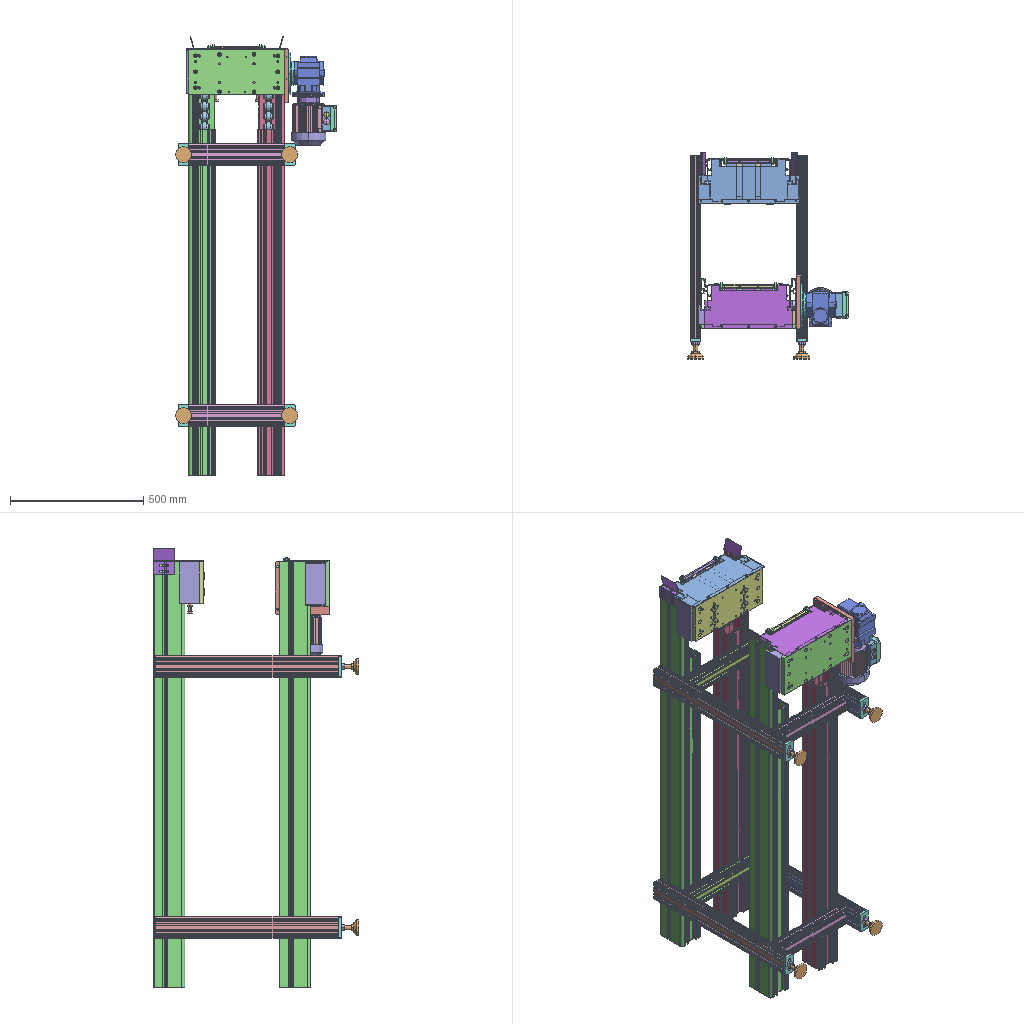Assembly | STEP file | 50 different items | 172 placed | box 603 x 771 x 1648 mm
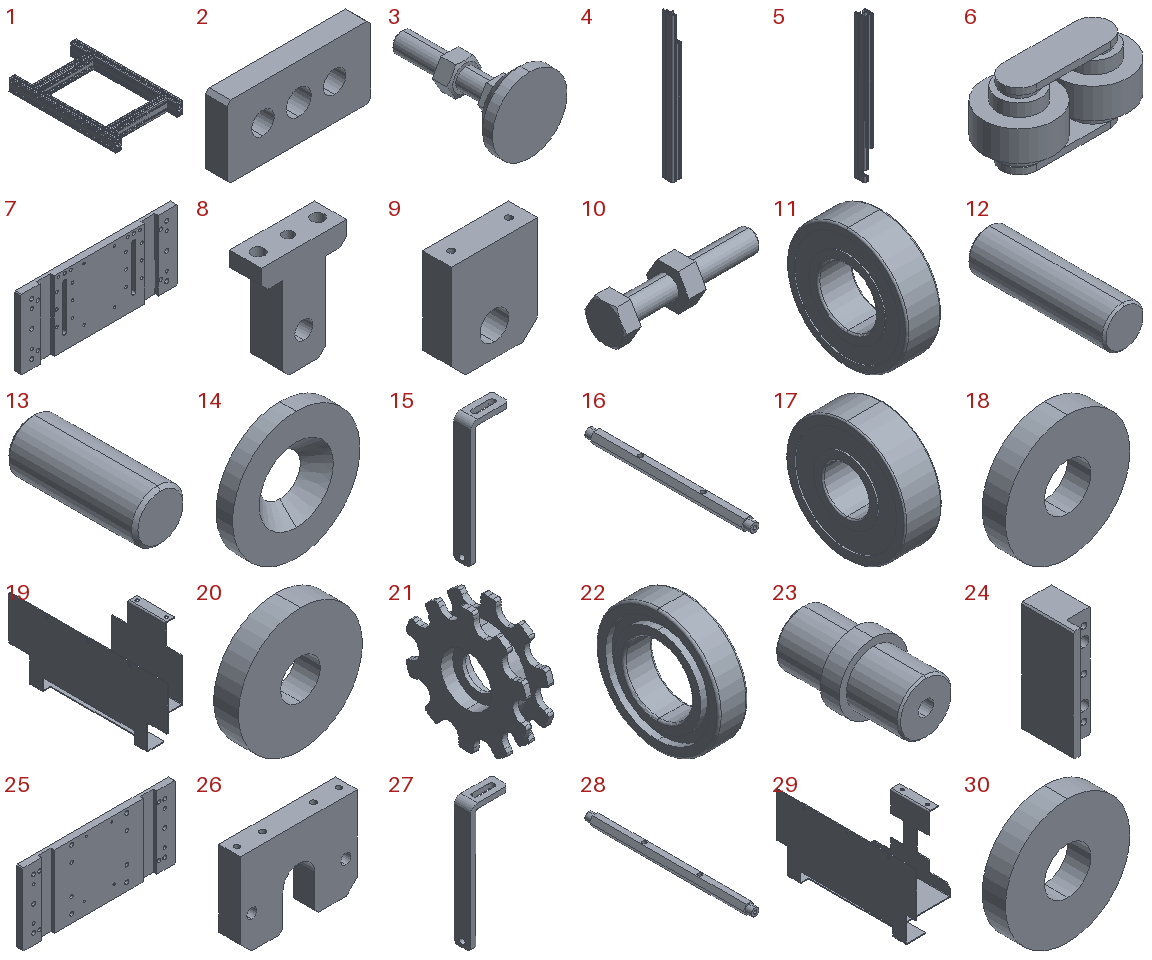Parts list (item | name | quantity | parent item | size | volume):
1 | - | x2 | - | 439.002 x 686.5 x 80 mm | 2058365 mm3
2 | - | x4 | - | 80 x 12 x 40 mm | 33512 mm3
3 | FJFN16-75_default | x4 | - | 60 x 103 x 60 mm | 66755 mm3
4 | - | x2 | - | 100 x 118 x 1600 mm | 2600704 mm3
5 | - | x2 | - | 100 x 118 x 1600 mm | 2582568 mm3
6 | PN_0025_default | x68 | - | 74.7 x 36.6 x 38.9 mm | 50379 mm3
7 | PN_0001_default | x1 | in PN_0015 | 359 x 15 x 160 mm | 723262 mm3
8 | PN_0002_default | x2 | in PN_0015 | 40 x 15 x 50 mm | 16009 mm3
9 | PN_0003_default | x2 | in PN_0015 | 90 x 30 x 105 mm | 254060 mm3
10 | M10-60_RCB10-70 | x2 | in PN_0015 | 67 x 19.63 x 17 mm | 7820 mm3
11 | bearingB6004ZZ_default | x1 | in B6004ZZ_B6004ZZ | 12 x 42 x 42 mm | 12378 mm3
12 | 6-20_default | x16 | in PN_0015 | 6 x 20 x 6 mm | 563.847 mm3
13 | 8-20_default | x4 | in PN_0015 | 8 x 20 x 8 mm | 999.288 mm3
14 | PN_0005_default | x5 | in PN_0015 | 38.5 x 5 x 38.5 mm | 4599 mm3
15 | PN_0006_default | x2 | in PN_0015 | 45 x 20 x 148 mm | 20804 mm3
16 | PN_0007_default | x1 | in PN_0015 | 13.856 x 185 x 12 mm | 21503 mm3
17 | B6000ZZ_B6000ZZ | x4 | in PN_0015, PN_0016 | 8 x 26 x 26 mm | 3459 mm3
18 | PN_0008_default | x2 | in PN_0015 | 16 x 3 x 16 mm | 518.363 mm3
19 | PN_0009_default | x1 | in PN_0015 | 162 x 379 x 167 mm | 195239 mm3
20 | PN_0010_default | x4 | in PN_0015 | 25 x 5 x 25 mm | 2203 mm3
21 | PN_0012_default | x2 | in PN_0015 | 30 x 129.474 x 133 mm | 166383 mm3
22 | B6006_B6006 | x4 | in PN_0015 | 13 x 55 x 55 mm | 18718 mm3
23 | PN_0004_default | x2 | in PN_0015 | 38 x 68.5 x 38 mm | 49766 mm3
24 | PN_0013_default | x3 | in PN_0015, PN_0016 | 44.75 x 75 x 160 mm | 399871 mm3
25 | PN_0017_default | x1 | in PN_0016 | 359 x 15 x 170 mm | 803822 mm3
26 | PN_0018_default | x2 | in PN_0016 | 161 x 30 x 120 mm | 471064 mm3
27 | PN_0020_default | x2 | in PN_0016 | 45 x 20 x 151 mm | 21164 mm3
28 | PN_0021_default | x1 | in PN_0016 | 13.856 x 210 x 12 mm | 24621 mm3
29 | PN_0022_default | x1 | in PN_0016 | 172 x 329 x 167 mm | 178980 mm3
30 | PN_0023_default | x2 | in PN_0016 | 16 x 3 x 16 mm | 518.363 mm3
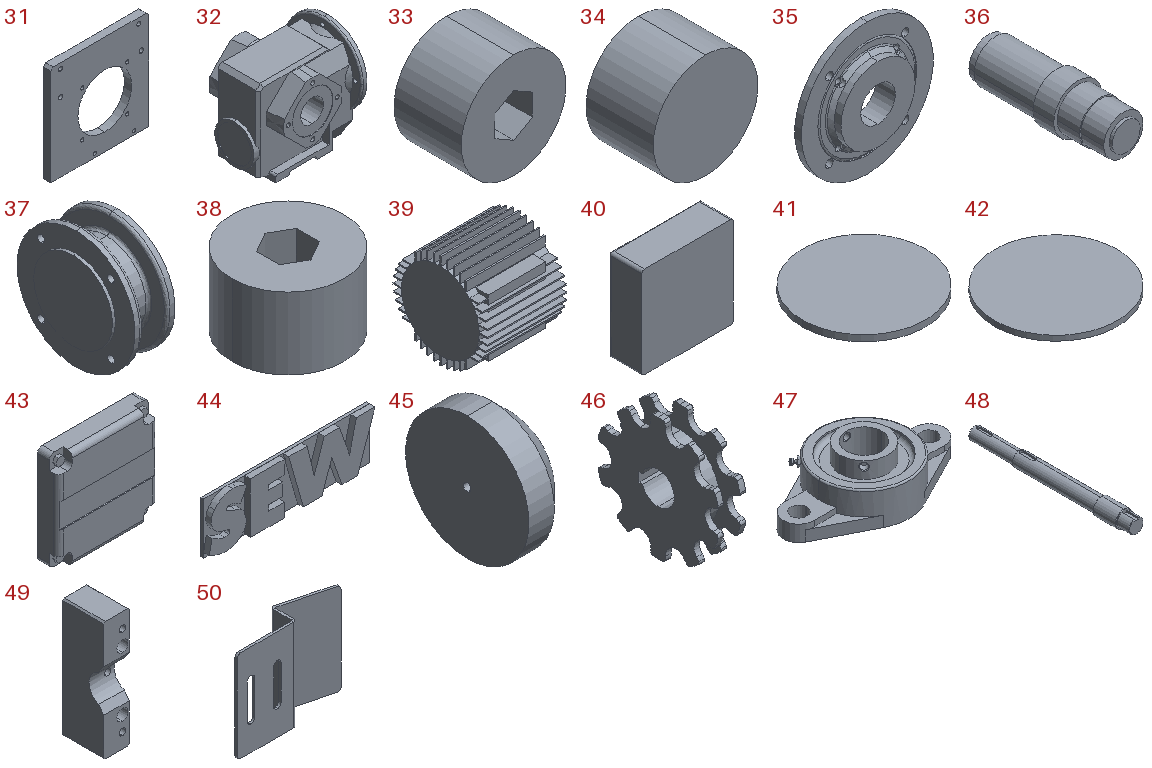31 | PN_0024_default | x1 | in PN_0016 | 200 x 15 x 203 mm | 456778 mm3
32 | PRODUCT_NAME_32_default | x1 | in SAF37DR63L4-TF-n104-M1-B | 143 x 120 x 142 mm | 1389830 mm3
33 | PRODUCT_NAME_33_default | x1 | in SAF37DR63L4-TF-n104-M1-B | 14 x 9 x 14 mm | 1299 mm3
34 | PRODUCT_NAME_34_default | x1 | in SAF37DR63L4-TF-n104-M1-B | 14 x 9 x 14 mm | 1299 mm3
35 | PRODUCT_NAME_35_default | x1 | in SAF37DR63L4-TF-n104-M1-B | 160 x 24 x 160 mm | 238568 mm3
36 | PRODUCT_NAME_36_default | x1 | in SAF37DR63L4-TF-n104-M1-B | 43 x 122.5 x 43 mm | 103084 mm3
37 | PRODUCT_NAME_37_default | x1 | in SAF37DR63L4-TF-n104-M1-B | 45 x 120 x 120 mm | 320577 mm3
38 | PRODUCT_NAME_38_default | x1 | in SAF37DR63L4-TF-n104-M1-B | 14 x 14 x 9 mm | 1299 mm3
39 | PRODUCT_NAME_39_default | x1 | in SAF37DR63L4-TF-n104-M1-B | 102 x 122 x 122 mm | 884304 mm3
40 | PRODUCT_NAME_40_default | x1 | in SAF37DR63L4-TF-n104-M1-B | 95 x 33 x 95 mm | 297490 mm3
41 | PRODUCT_NAME_41_default | x1 | in SAF37DR63L4-TF-n104-M1-B | 20 x 20 x 3.972 mm | 728.684 mm3
42 | PRODUCT_NAME_42_default | x1 | in SAF37DR63L4-TF-n104-M1-B | 24 x 24 x 4.478 mm | 1175 mm3
43 | PRODUCT_NAME_43_default | x1 | in SAF37DR63L4-TF-n104-M1-B | 100 x 21.5 x 100 mm | 204377 mm3
44 | PRODUCT_NAME_44_default | x1 | in SAF37DR63L4-TF-n104-M1-B | 58.086 x 3 x 18.091 mm | 2435 mm3
45 | PRODUCT_NAME_45_default | x1 | in SAF37DR63L4-TF-n104-M1-B | 47 x 132 x 132 mm | 566262 mm3
46 | PN_0011_default | x2 | in PN_0016 | 30 x 129.474 x 133 mm | 202077 mm3
47 | HDH35_HDH35 | x2 | in PN_0016 | 161 x 90 x 44.4 mm | 197699 mm3
48 | PN_0019_default | x1 | in PN_0016 | 42 x 401.5 x 42 mm | 377552 mm3
49 | PN_0014_default | x1 | in PN_0016 | 34 x 55 x 160 mm | 251328 mm3
50 | - | x2 | - | 98.296 x 21.17 x 80 mm | 17841 mm3
Placements (level | parent | child | x y z in mm | rotation matrix by rows):
1 | subassembly 2 | subassembly 3 | -225.021 25.346 -0.0 | 1 0 0 0 1 0 0 0 1
2 | subassembly 3 | subassembly 4 | -223.832 -352.823 20.0 | 1 0 0 0 1 0 0 0 1
2 | subassembly 3 | subassembly 5 | -223.832 -364.823 0.0 | 0 0 1 0 1 0 -1 0 0
2 | subassembly 3 | FJFN16-75_default | -223.832 -429.323 0.0 | 1 0 0 0 1 0 0 0 1
2 | subassembly 3 | FJFN16-75_default | 175.168 -429.323 0.0 | -1 0 0 0 1 0 0 0 -1
2 | subassembly 3 | subassembly 5 | 175.168 -364.823 0.0 | 0 0 1 0 1 0 -1 0 0
1 | subassembly 2 | subassembly 6 | -9538.032 1852.311 -225.0 | 1 0 0 0 1 0 0 0 1
1 | subassembly 2 | subassembly 7 | 9039.328 1852.311 1375.0 | -1 0 0 0 1 0 0 0 -1
1 | subassembly 2 | subassembly 3 | -225.021 25.346 980.0 | 1 0 0 0 1 0 0 0 1
2 | subassembly 3 | subassembly 4 | -223.832 -352.823 20.0 | 1 0 0 0 1 0 0 0 1
2 | subassembly 3 | subassembly 5 | -223.832 -364.823 0.0 | 0 0 1 0 1 0 -1 0 0
2 | subassembly 3 | FJFN16-75_default | -223.832 -429.323 0.0 | 1 0 0 0 1 0 0 0 1
2 | subassembly 3 | FJFN16-75_default | 175.168 -429.323 0.0 | -1 0 0 0 1 0 0 0 -1
2 | subassembly 3 | subassembly 5 | 175.168 -364.823 0.0 | 0 0 1 0 1 0 -1 0 0
1 | subassembly 2 | PN_0025_default | -148.802 329.638 -165.0 | 0 0 1 0 1 0 -1 0 0
1 | subassembly 2 | PN_0025_default | -148.802 329.638 -87.0 | 0 0 1 0 1 0 -1 0 0
1 | subassembly 2 | PN_0025_default | -148.802 329.638 -9.0 | 0 0 1 0 1 0 -1 0 0
1 | subassembly 2 | PN_0025_default | -148.802 329.638 69.0 | 0 0 1 0 1 0 -1 0 0
1 | subassembly 2 | PN_0025_default | -148.802 329.638 147.0 | 0 0 1 0 1 0 -1 0 0
1 | subassembly 2 | PN_0025_default | -148.802 329.638 225.0 | 0 0 1 0 1 0 -1 0 0
1 | subassembly 2 | PN_0025_default | -148.802 329.638 303.0 | 0 0 1 0 1 0 -1 0 0
1 | subassembly 2 | PN_0025_default | -148.802 329.638 381.0 | 0 0 1 0 1 0 -1 0 0
1 | subassembly 2 | PN_0025_default | -148.802 329.638 459.0 | 0 0 1 0 1 0 -1 0 0
1 | subassembly 2 | PN_0025_default | -148.802 329.638 537.0 | 0 0 1 0 1 0 -1 0 0
1 | subassembly 2 | PN_0025_default | -148.802 329.638 615.0 | 0 0 1 0 1 0 -1 0 0
1 | subassembly 2 | PN_0025_default | -148.802 329.638 693.0 | 0 0 1 0 1 0 -1 0 0
1 | subassembly 2 | PN_0025_default | -148.802 329.638 771.0 | 0 0 1 0 1 0 -1 0 0
1 | subassembly 2 | PN_0025_default | -148.802 329.638 849.0 | 0 0 1 0 1 0 -1 0 0
1 | subassembly 2 | PN_0025_default | -148.802 329.638 927.0 | 0 0 1 0 1 0 -1 0 0
1 | subassembly 2 | PN_0025_default | -148.802 329.638 1005.0 | 0 0 1 0 1 0 -1 0 0
1 | subassembly 2 | PN_0025_default | -148.802 329.638 1083.0 | 0 0 1 0 1 0 -1 0 0
1 | subassembly 2 | PN_0025_default | -148.802 329.638 1161.0 | 0 0 1 0 1 0 -1 0 0
1 | subassembly 2 | PN_0025_default | -148.802 329.638 1239.0 | 0 0 1 0 1 0 -1 0 0
1 | subassembly 2 | PN_0025_default | -148.802 329.638 1317.0 | 0 0 1 0 1 0 -1 0 0
1 | subassembly 2 | PN_0025_default | -388.802 329.638 -165.0 | 0 0 1 0 1 0 -1 0 0
1 | subassembly 2 | PN_0025_default | -388.802 329.638 -87.0 | 0 0 1 0 1 0 -1 0 0
1 | subassembly 2 | PN_0025_default | -388.802 329.638 -9.0 | 0 0 1 0 1 0 -1 0 0
1 | subassembly 2 | PN_0025_default | -388.802 329.638 1317.0 | 0 0 1 0 1 0 -1 0 0
1 | subassembly 2 | PN_0025_default | -388.802 329.638 69.0 | 0 0 1 0 1 0 -1 0 0
1 | subassembly 2 | PN_0025_default | -388.802 329.638 147.0 | 0 0 1 0 1 0 -1 0 0
1 | subassembly 2 | PN_0025_default | -388.802 329.638 225.0 | 0 0 1 0 1 0 -1 0 0
1 | subassembly 2 | PN_0025_default | -388.802 329.638 303.0 | 0 0 1 0 1 0 -1 0 0
1 | subassembly 2 | PN_0025_default | -388.802 329.638 381.0 | 0 0 1 0 1 0 -1 0 0
1 | subassembly 2 | PN_0025_default | -388.802 329.638 459.0 | 0 0 1 0 1 0 -1 0 0
1 | subassembly 2 | PN_0025_default | -388.802 329.638 537.0 | 0 0 1 0 1 0 -1 0 0
1 | subassembly 2 | PN_0025_default | -388.802 329.638 615.0 | 0 0 1 0 1 0 -1 0 0
1 | subassembly 2 | PN_0025_default | -388.802 329.638 693.0 | 0 0 1 0 1 0 -1 0 0
1 | subassembly 2 | PN_0025_default | -388.802 329.638 771.0 | 0 0 1 0 1 0 -1 0 0
1 | subassembly 2 | PN_0025_default | -388.802 329.638 849.0 | 0 0 1 0 1 0 -1 0 0
1 | subassembly 2 | PN_0025_default | -388.802 329.638 927.0 | 0 0 1 0 1 0 -1 0 0
1 | subassembly 2 | PN_0025_default | -388.802 329.638 1005.0 | 0 0 1 0 1 0 -1 0 0
1 | subassembly 2 | PN_0025_default | -388.802 329.638 1083.0 | 0 0 1 0 1 0 -1 0 0
1 | subassembly 2 | PN_0025_default | -388.802 329.638 1161.0 | 0 0 1 0 1 0 -1 0 0
1 | subassembly 2 | PN_0025_default | -388.802 329.638 1239.0 | 0 0 1 0 1 0 -1 0 0
1 | subassembly 2 | PN_0015 | -251.774 212.504 1295.0 | 1 0 0 0 -1 0 0 0 -1
2 | PN_0015 | PN_0001_default | 2.422 18.481 -0.0 | 1 0 0 0 1 0 0 0 1
2 | PN_0015 | PN_0002_default | -76.828 -6.519 80.0 | 1 0 0 0 0 1 0 -1 -0
2 | PN_0015 | PN_0002_default | 81.672 -6.519 80.0 | 1 0 0 0 0 1 0 -1 -0
2 | PN_0015 | PN_0003_default | -76.828 -34.019 5.0 | 0 1 0 0 0 1 1 0 -0
2 | PN_0015 | PN_0003_default | 81.672 -34.019 5.0 | 0 -1 0 0 0 1 -1 0 -0
2 | PN_0015 | M10-60_RCB10-70 | 81.672 -16.519 110.0 | 0 0.5 0.866 0 0.866 -0.5 -1 0 -0
2 | PN_0015 | M10-60_RCB10-70 | -76.828 -16.519 110.0 | 0 0.5 0.866 0 0.866 -0.5 -1 0 0
2 | PN_0015 | B6004ZZ_B6004ZZ | -76.828 -61.519 0.0 | 1 0 0 0 1 0 0 0 1
3 | B6004ZZ_B6004ZZ | bearingB6004ZZ_default | -0.0 0.0 -0.0 | 1 0 0 0 1 0 0 0 1
2 | PN_0015 | 6-20_default | -58.828 8.481 45.0 | 1 0 0 0 1 0 0 0 1
2 | PN_0015 | 6-20_default | -58.828 8.481 10.0 | 1 0 0 0 1 0 0 0 1
2 | PN_0015 | 6-20_default | -58.828 8.481 -25.0 | 1 0 0 0 1 0 0 0 1
2 | PN_0015 | 6-20_default | -94.828 8.481 45.0 | 0.1404 0 0.9901 0 1 0 -0.9901 0 0.1404
2 | PN_0015 | 6-20_default | -94.828 8.481 10.0 | 1 0 0 0 1 0 0 0 1
2 | PN_0015 | 6-20_default | -94.828 8.481 -25.0 | 1 0 0 0 1 0 0 0 1
2 | PN_0015 | 6-20_default | -62.828 8.481 72.5 | 1 0 0 0 1 0 0 0 1
2 | PN_0015 | 6-20_default | -90.828 8.481 72.5 | 1 0 0 0 1 0 0 0 1
2 | PN_0015 | 6-20_default | 95.672 8.481 72.5 | 0.9561 0 -0.2931 0 1 0 0.2931 0 0.9561
2 | PN_0015 | 6-20_default | 67.672 8.481 72.5 | 0.9667 0 -0.2559 0 1 0 0.2559 0 0.9667
2 | PN_0015 | 6-20_default | 99.672 8.481 45.0 | 0.4544 0 -0.8908 0 1 0 0.8908 0 0.4544
2 | PN_0015 | 6-20_default | 99.672 8.481 10.0 | 1 0 0 0 1 0 0 0 1
2 | PN_0015 | 6-20_default | 99.672 8.481 -25.0 | 1 0 0 0 1 0 0 0 1
2 | PN_0015 | 6-20_default | 63.672 8.481 45.0 | 1 0 0 0 1 0 0 0 1
2 | PN_0015 | 6-20_default | 63.672 8.481 10.0 | 1 0 0 0 1 0 0 0 1
2 | PN_0015 | 6-20_default | 63.672 8.481 -25.0 | 1 0 0 0 1 0 0 0 1
2 | PN_0015 | 8-20_default | 143.172 8.481 -50.0 | 1 0 0 0 1 0 0 0 1
2 | PN_0015 | 8-20_default | 143.172 8.481 50.0 | 1 0 0 0 1 0 0 0 1
2 | PN_0015 | 8-20_default | -138.328 8.481 50.0 | 0.2064 0 -0.9785 0 1 0 0.9785 0 0.2064
2 | PN_0015 | 8-20_default | -138.328 8.481 -50.0 | 1 0 0 0 1 0 0 0 1
2 | PN_0015 | PN_0005_default | -59.828 -61.519 0.0 | 0 -1 0 -0.3818 0 -0.9242 0.9242 0 -0.3818
2 | PN_0015 | PN_0006_default | 27.422 -55.519 -55.5 | 0 1 0 0 0 1 1 0 -0
2 | PN_0015 | PN_0006_default | -42.578 -55.519 -55.5 | 0 1 0 0 0 1 1 0 -0
2 | PN_0015 | PN_0007_default | -90.078 -123.519 -84.0 | 0 1 0 -1 0 0 0 0 1
2 | PN_0015 | B6000ZZ_B6000ZZ | 94.922 -123.519 -84.0 | -1 0 0 0 -1 0 0 0 1
2 | PN_0015 | B6000ZZ_B6000ZZ | -82.078 -123.519 -84.0 | -1 0 0 0 -0.8372 0.5469 0 0.5469 0.8372
2 | PN_0015 | PN_0008_default | 94.922 -123.519 -84.0 | 0 1 0 -0.9644 0 -0.2646 -0.2646 0 0.9644
2 | PN_0015 | PN_0008_default | -90.078 -123.519 -84.0 | 0 -1 0 0.8671 0 0.4981 -0.4981 0 0.8671
2 | PN_0015 | PN_0009_default | -137.578 33.481 -80.0 | 0 1 0 0 0 1 1 0 0
2 | PN_0015 | PN_0010_default | 81.672 33.481 -25.0 | 1 0 0 0 1 0 0 0 1
2 | PN_0015 | PN_0010_default | 81.672 33.481 35.0 | 1 0 0 0 1 0 0 0 1
2 | PN_0015 | PN_0010_default | -76.828 33.481 -25.0 | 1 0 0 0 1 0 0 0 1
2 | PN_0015 | PN_0010_default | -76.828 33.481 35.0 | 1 0 0 0 1 0 0 0 1
2 | PN_0015 | PN_0012_default | 107.172 -56.519 5.0 | 1 0 0 0 0.9423 0.3348 0 -0.3348 0.9423
2 | PN_0015 | B6006_B6006 | 124.172 -56.519 5.0 | 1 0 0 0 0.9955 -0.09481 0 0.09481 0.9955
2 | PN_0015 | B6006_B6006 | 107.172 -56.519 5.0 | 1 0 0 0 0.9955 -0.09481 0 0.09481 0.9955
2 | PN_0015 | PN_0004_default | 107.172 -56.519 5.0 | 0 -1 0 0.9968 0 -0.08002 0.08002 0 0.9968
2 | PN_0015 | PN_0005_default | 61.672 -56.519 5.0 | 0 1 0 -0.3818 0 0.9242 0.9242 0 0.3818
2 | PN_0015 | PN_0005_default | 142.172 -56.519 5.0 | 0 -1 0 0.5523 0 0.8337 -0.8337 0 0.5523
2 | PN_0015 | PN_0005_default | -137.328 -56.519 5.0 | 0 1 0 0.5523 0 -0.8337 -0.8337 0 -0.5523
2 | PN_0015 | PN_0012_default | -102.328 -56.519 5.0 | -1 0 0 0 0.9423 -0.3348 0 -0.3348 -0.9423
2 | PN_0015 | PN_0004_default | -102.328 -56.519 5.0 | 0 1 0 0.9968 0 0.08002 0.08002 0 -0.9968
2 | PN_0015 | B6006_B6006 | -102.328 -56.519 5.0 | -1 0 0 0 0.9955 0.09481 0 0.09481 -0.9955
2 | PN_0015 | B6006_B6006 | -119.328 -56.519 5.0 | -1 0 0 0 0.9955 0.09481 0 0.09481 -0.9955
2 | PN_0015 | PN_0005_default | -56.828 -56.519 5.0 | 0 -1 0 -0.3818 0 -0.9242 0.9242 0 -0.3818
2 | PN_0015 | PN_0013_default | -164.703 -56.519 -0.0 | 1 0 0 0 1 0 0 0 1
2 | PN_0015 | PN_0013_default | 169.547 -56.519 -0.0 | -1 0 0 0 1 0 0 0 -1
1 | subassembly 2 | PN_0025_default | -148.802 -142.362 -165.0 | 0 0 1 0 1 0 -1 0 0
1 | subassembly 2 | PN_0025_default | -148.802 -142.362 -9.0 | 0 0 1 0 1 0 -1 0 0
1 | subassembly 2 | PN_0025_default | -148.802 -142.362 -87.0 | 0 0 1 0 1 0 -1 0 0
1 | subassembly 2 | PN_0025_default | -388.802 -142.362 69.0 | 0 0 1 0 1 0 -1 0 0
1 | subassembly 2 | PN_0025_default | -388.802 -142.362 -9.0 | 0 0 1 0 1 0 -1 0 0
1 | subassembly 2 | PN_0025_default | -388.802 -142.362 -87.0 | 0 0 1 0 1 0 -1 0 0
1 | subassembly 2 | PN_0025_default | -388.802 -142.362 -165.0 | 0 0 1 0 1 0 -1 0 0
1 | subassembly 2 | subassembly 7 | 9039.328 1380.311 1375.0 | -1 0 0 0 1 0 0 0 -1
1 | subassembly 2 | subassembly 6 | -9538.032 1380.311 -225.0 | 1 0 0 0 1 0 0 0 1
1 | subassembly 2 | PN_0025_default | -388.802 -142.362 771.0 | 0 0 1 0 1 0 -1 0 0
1 | subassembly 2 | PN_0025_default | -388.802 -142.362 693.0 | 0 0 1 0 1 0 -1 0 0
1 | subassembly 2 | PN_0025_default | -388.802 -142.362 381.0 | 0 0 1 0 1 0 -1 0 0
1 | subassembly 2 | PN_0025_default | -388.802 -142.362 459.0 | 0 0 1 0 1 0 -1 0 0
1 | subassembly 2 | PN_0025_default | -388.802 -142.362 537.0 | 0 0 1 0 1 0 -1 0 0
1 | subassembly 2 | PN_0025_default | -388.802 -142.362 615.0 | 0 0 1 0 1 0 -1 0 0
1 | subassembly 2 | PN_0025_default | -148.802 -142.362 381.0 | 0 0 1 0 1 0 -1 0 0
1 | subassembly 2 | PN_0025_default | -148.802 -142.362 459.0 | 0 0 1 0 1 0 -1 0 0
1 | subassembly 2 | PN_0025_default | -148.802 -142.362 537.0 | 0 0 1 0 1 0 -1 0 0
1 | subassembly 2 | PN_0025_default | -148.802 -142.362 615.0 | 0 0 1 0 1 0 -1 0 0
1 | subassembly 2 | PN_0025_default | -148.802 -142.362 693.0 | 0 0 1 0 1 0 -1 0 0
1 | subassembly 2 | PN_0025_default | -148.802 -142.362 771.0 | 0 0 1 0 1 0 -1 0 0
1 | subassembly 2 | PN_0025_default | -148.802 -142.362 849.0 | 0 0 1 0 1 0 -1 0 0
1 | subassembly 2 | PN_0016 | -265.491 -254.431 1290.0 | 1 0 0 0 -1 0 0 0 -1
2 | PN_0016 | PN_0017_default | 16.139 23.546 0.0 | 1 0 0 0 1 0 0 0 1
2 | PN_0016 | PN_0018_default | -63.861 -36.454 4.5 | 0 1 0 0 0 1 1 0 -0
2 | PN_0016 | PN_0018_default | 96.139 -36.454 4.5 | 0 -1 0 0 0 1 -1 0 0
2 | PN_0016 | PN_0020_default | -28.861 -51.954 -57.5 | 0 1 0 0 0 1 1 0 -0
2 | PN_0016 | PN_0020_default | 41.139 -51.954 -57.5 | 0 1 0 0 0 1 1 0 -0
2 | PN_0016 | PN_0021_default | -88.861 -121.454 -86.0 | 0 1 0 -1 0 0 0 0 1
2 | PN_0016 | B6000ZZ_B6000ZZ | -88.861 -121.454 -86.0 | 1 0 0 0 0 -1 0 1 -0
2 | PN_0016 | B6000ZZ_B6000ZZ | 113.139 -121.454 -86.0 | 1 0 0 0 0.9207 0.3904 0 -0.3904 0.9207
2 | PN_0016 | PN_0022_default | -124.361 38.546 -85.0 | 0 1 0 0 0 1 1 0 -0
2 | PN_0016 | PN_0023_default | -88.861 -121.454 -86.0 | 0 -1 0 0.922 0 -0.3872 0.3872 0 0.922
2 | PN_0016 | PN_0023_default | 121.139 -121.454 -86.0 | 0 1 0 -0.879 0 0.4768 0.4768 0 0.879
2 | PN_0016 | PN_0024_default | 195.639 -67.954 15.0 | 0 1 0 0 0 -1 -1 0 -0
2 | PN_0016 | SAF37DR63L4-TF-n104-M1-B | 342.639 -51.454 4.5 | 0 -1 0 0 0 -1 1 0 -0
3 | SAF37DR63L4-TF-n104-M1-B | PRODUCT_NAME_32_default | -0.0 0.0 0.0 | 1 0 0 0 1 0 0 0 1
3 | SAF37DR63L4-TF-n104-M1-B | PRODUCT_NAME_33_default | -0.0 0.0 0.0 | 1 0 0 0 1 0 0 0 1
3 | SAF37DR63L4-TF-n104-M1-B | PRODUCT_NAME_34_default | -0.0 0.0 0.0 | 1 0 0 0 1 0 0 0 1
3 | SAF37DR63L4-TF-n104-M1-B | PRODUCT_NAME_35_default | -0.0 0.0 0.0 | 1 0 0 0 1 0 0 0 1
3 | SAF37DR63L4-TF-n104-M1-B | PRODUCT_NAME_36_default | -0.0 0.0 0.0 | 1 0 0 0 1 0 0 0 1
3 | SAF37DR63L4-TF-n104-M1-B | PRODUCT_NAME_37_default | -0.0 16.695 40.305 | 1 0 0 0 0.7071 0.7071 0 -0.7071 0.7071
3 | SAF37DR63L4-TF-n104-M1-B | PRODUCT_NAME_38_default | -0.0 0.0 0.0 | 1 0 0 0 1 0 0 0 1
3 | SAF37DR63L4-TF-n104-M1-B | PRODUCT_NAME_39_default | -0.0 0.0 0.0 | 1 0 0 0 1 0 0 0 1
3 | SAF37DR63L4-TF-n104-M1-B | PRODUCT_NAME_40_default | -0.0 0.0 0.0 | 1 0 0 0 1 0 0 0 1
3 | SAF37DR63L4-TF-n104-M1-B | PRODUCT_NAME_41_default | -0.0 0.0 0.0 | 1 0 0 0 1 0 0 0 1
3 | SAF37DR63L4-TF-n104-M1-B | PRODUCT_NAME_42_default | -0.0 0.0 0.0 | 1 0 0 0 1 0 0 0 1
3 | SAF37DR63L4-TF-n104-M1-B | PRODUCT_NAME_43_default | -0.0 0.0 0.0 | 1 0 0 0 1 0 0 0 1
3 | SAF37DR63L4-TF-n104-M1-B | PRODUCT_NAME_44_default | -0.0 0.0 0.0 | 1 0 0 0 1 0 0 0 1
3 | SAF37DR63L4-TF-n104-M1-B | PRODUCT_NAME_45_default | -0.0 0.0 0.0 | 1 0 0 0 1 0 0 0 1
2 | PN_0016 | PN_0011_default | -118.861 -51.454 4.5 | 1 0 0 0 0.5222 0.8529 0 -0.8529 0.5222
2 | PN_0016 | PN_0011_default | 151.139 -51.454 4.5 | -1 0 0 0 0.5222 -0.8529 0 -0.8529 -0.5222
2 | PN_0016 | HDH35_HDH35 | -11.661 -51.454 4.5 | 0 0 1 0 1 0 -1 0 -0
2 | PN_0016 | HDH35_HDH35 | 43.939 -51.415 4.5 | 0 0 -1 0 -1 0 -1 0 -0
2 | PN_0016 | PN_0019_default | -118.861 -51.454 4.5 | 0 1 0 0.8529 0 0.5222 0.5222 0 -0.8529
2 | PN_0016 | PN_0013_default | -150.986 -51.454 0.0 | 1 0 0 0 1 0 0 0 1
2 | PN_0016 | PN_0014_default | 178.639 -31.454 -0.0 | -1 0 0 0 1 0 0 0 -1
1 | subassembly 2 | PN_0025_default | -148.802 -142.362 1083.0 | 0 0 1 0 1 0 -1 0 0
1 | subassembly 2 | PN_0025_default | -388.802 -142.362 1083.0 | 0 0 1 0 1 0 -1 0 0
1 | subassembly 2 | PN_0025_default | -388.802 -142.362 1161.0 | 0 0 1 0 1 0 -1 0 0
1 | subassembly 2 | PN_0025_default | -388.802 -142.362 1239.0 | 0 0 1 0 1 0 -1 0 0
1 | subassembly 2 | PN_0025_default | -388.802 -142.362 1317.0 | 0 0 1 0 1 0 -1 0 0
1 | subassembly 2 | PN_0025_default | -148.802 -142.362 1161.0 | 0 0 1 0 1 0 -1 0 0
1 | subassembly 2 | PN_0025_default | -148.802 -142.362 1239.0 | 0 0 1 0 1 0 -1 0 0
1 | subassembly 2 | PN_0025_default | -148.802 -142.362 1317.0 | 0 0 1 0 1 0 -1 0 0
1 | subassembly 2 | subassembly 8 | -428.852 287.023 1325.0 | 0 1 0 0 0 1 1 0 -0
1 | subassembly 2 | subassembly 8 | -69.852 367.023 1325.0 | 0 -1 0 0 0 -1 1 0 -0